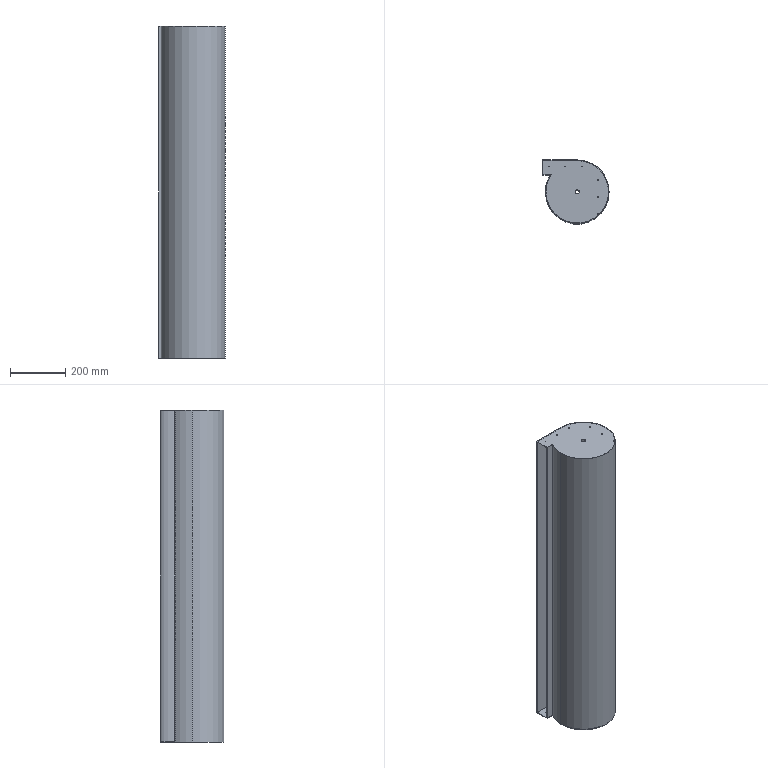Part | SolidWorks | features BaseBody 1 | 1 solid | 43 faces | box 239.936 x 230.88 x 1204 mm | volume 2000614 mm3 | cylinder 34 | plane 9 | commonest cylinder face diameters 3.455 x24 15 x4 226.88 x3 230.88 x3
STEP:
#1=CARTESIAN_POINT('',(74.043,-287.472,-1202.));
#2=VERTEX_POINT('',#1);
#3=CARTESIAN_POINT('',(56.063,-349.342,-1202.));
#4=VERTEX_POINT('',#3);
#5=CARTESIAN_POINT('',(171.503,-349.342,-1202.));
#6=DIRECTION('',(0.,0.,1.));
#7=DIRECTION('',(1.,0.,0.));
#8=AXIS2_PLACEMENT_3D('',#5,#6,#7);
#9=CIRCLE('',#8,115.44);
#10=EDGE_CURVE('',#2,#4,#9,.T.);
#11=ORIENTED_EDGE('',*,*,#10,.T.);
#12=CARTESIAN_POINT('',(56.063,-349.342,2.));
#13=VERTEX_POINT('',#12);
#14=CARTESIAN_POINT('',(56.063,-349.342,0.));
#15=DIRECTION('',(0.,0.,1.));
#16=VECTOR('',#15,1000.);
#17=LINE('',#14,#16);
#18=EDGE_CURVE('',#4,#13,#17,.T.);
#19=ORIENTED_EDGE('',*,*,#18,.T.);
#20=CARTESIAN_POINT('',(74.043,-287.472,2.));
#21=VERTEX_POINT('',#20);
#22=CARTESIAN_POINT('',(171.503,-349.342,2.));
#23=DIRECTION('',(0.,0.,-1.));
#24=DIRECTION('',(1.,0.,0.));
#25=AXIS2_PLACEMENT_3D('',#22,#23,#24);
#26=CIRCLE('',#25,115.44);
#27=EDGE_CURVE('',#13,#21,#26,.T.);
#28=ORIENTED_EDGE('',*,*,#27,.T.);
#29=CARTESIAN_POINT('',(74.043,-287.472,0.));
#30=DIRECTION('',(0.,0.,-1.));
#31=VECTOR('',#30,1000.);
#32=LINE('',#29,#31);
#33=EDGE_CURVE('',#21,#2,#32,.T.);
#34=ORIENTED_EDGE('',*,*,#33,.T.);
#35=EDGE_LOOP('',(#11,#19,#28,#34));
#36=FACE_OUTER_BOUND('',#35,.T.);
#37=CARTESIAN_POINT('',(171.503,-349.342,0.));
#38=DIRECTION('',(0.,0.,1.));
#39=DIRECTION('',(1.,0.,0.));
#40=AXIS2_PLACEMENT_3D('',#37,#38,#39);
#41=CYLINDRICAL_SURFACE('',#40,115.44);
#42=ADVANCED_FACE('',(#36),#41,.T.);
#43=ORIENTED_EDGE('',*,*,#18,.F.);
#44=CARTESIAN_POINT('',(286.943,-349.342,-1202.));
#45=VERTEX_POINT('',#44);
#46=CARTESIAN_POINT('',(171.503,-349.342,-1202.));
#47=DIRECTION('',(0.,0.,1.));
#48=DIRECTION('',(1.,0.,0.));
#49=AXIS2_PLACEMENT_3D('',#46,#47,#48);
#50=CIRCLE('',#49,115.44);
#51=EDGE_CURVE('',#4,#45,#50,.T.);
#52=ORIENTED_EDGE('',*,*,#51,.T.);
#53=CARTESIAN_POINT('',(286.943,-349.342,2.));
#54=VERTEX_POINT('',#53);
#55=CARTESIAN_POINT('',(286.943,-349.342,0.));
#56=DIRECTION('',(0.,0.,1.));
#57=VECTOR('',#56,1000.);
#58=LINE('',#55,#57);
#59=EDGE_CURVE('',#45,#54,#58,.T.);
#60=ORIENTED_EDGE('',*,*,#59,.T.);
#61=CARTESIAN_POINT('',(171.503,-349.342,2.));
#62=DIRECTION('',(0.,0.,-1.));
#63=DIRECTION('',(1.,0.,0.));
#64=AXIS2_PLACEMENT_3D('',#61,#62,#63);
#65=CIRCLE('',#64,115.44);
#66=EDGE_CURVE('',#54,#13,#65,.T.);
#67=ORIENTED_EDGE('',*,*,#66,.T.);
#68=EDGE_LOOP('',(#43,#52,#60,#67));
#69=FACE_OUTER_BOUND('',#68,.T.);
#70=CARTESIAN_POINT('',(171.503,-349.342,0.));
#71=DIRECTION('',(0.,0.,1.));
#72=DIRECTION('',(1.,0.,0.));
#73=AXIS2_PLACEMENT_3D('',#70,#71,#72);
#74=CYLINDRICAL_SURFACE('',#73,115.44);
#75=ADVANCED_FACE('',(#69),#74,.T.);
#76=CARTESIAN_POINT('',(179.003,-349.342,-1202.));
#77=VERTEX_POINT('',#76);
#78=CARTESIAN_POINT('',(164.003,-349.342,-1202.));
#79=VERTEX_POINT('',#78);
#80=CARTESIAN_POINT('',(171.503,-349.342,-1202.));
#81=DIRECTION('',(0.,0.,-1.));
#82=DIRECTION('',(1.,0.,0.));
#83=AXIS2_PLACEMENT_3D('',#80,#81,#82);
#84=CIRCLE('',#83,7.5);
#85=EDGE_CURVE('',#77,#79,#84,.T.);
#86=ORIENTED_EDGE('',*,*,#85,.T.);
#87=CARTESIAN_POINT('',(164.003,-349.342,-1200.));
#88=VERTEX_POINT('',#87);
#89=CARTESIAN_POINT('',(164.003,-349.342,-1202.));
#90=DIRECTION('',(0.,0.,1.));
#91=VECTOR('',#90,1000.);
#92=LINE('',#89,#91);
#93=EDGE_CURVE('',#79,#88,#92,.T.);
#94=ORIENTED_EDGE('',*,*,#93,.T.);
#95=CARTESIAN_POINT('',(179.003,-349.342,-1200.));
#96=VERTEX_POINT('',#95);
#97=CARTESIAN_POINT('',(171.503,-349.342,-1200.));
#98=DIRECTION('',(0.,0.,-1.));
#99=DIRECTION('',(1.,0.,0.));
#100=AXIS2_PLACEMENT_3D('',#97,#98,#99);
#101=CIRCLE('',#100,7.5);
#102=EDGE_CURVE('',#96,#88,#101,.T.);
#103=ORIENTED_EDGE('',*,*,#102,.F.);
#104=CARTESIAN_POINT('',(179.003,-349.342,-1202.));
#105=DIRECTION('',(0.,0.,1.));
#106=VECTOR('',#105,1000.);
#107=LINE('',#104,#106);
#108=EDGE_CURVE('',#77,#96,#107,.T.);
#109=ORIENTED_EDGE('',*,*,#108,.F.);
#110=EDGE_LOOP('',(#86,#94,#103,#109));
#111=FACE_OUTER_BOUND('',#110,.T.);
#112=CARTESIAN_POINT('',(171.503,-349.342,-1202.));
#113=DIRECTION('',(0.,0.,1.));
#114=DIRECTION('',(1.,0.,0.));
#115=AXIS2_PLACEMENT_3D('',#112,#113,#114);
#116=CYLINDRICAL_SURFACE('',#115,7.5);
#117=ADVANCED_FACE('',(#111),#116,.F.);
#118=CARTESIAN_POINT('',(248.518,-430.281,-1200.));
#119=VERTEX_POINT('',#118);
#120=CARTESIAN_POINT('',(245.063,-430.281,-1200.));
#121=VERTEX_POINT('',#120);
#122=CARTESIAN_POINT('',(246.79,-430.281,-1200.));
#123=DIRECTION('',(0.,0.,-1.));
#124=DIRECTION('',(-1.,0.,0.));
#125=AXIS2_PLACEMENT_3D('',#122,#123,#124);
#126=CIRCLE('',#125,1.728);
#127=EDGE_CURVE('',#119,#121,#126,.T.);
#128=ORIENTED_EDGE('',*,*,#127,.F.);
#129=CARTESIAN_POINT('',(248.518,-430.281,-1202.));
#130=VERTEX_POINT('',#129);
#131=CARTESIAN_POINT('',(248.518,-430.281,2.));
#132=DIRECTION('',(0.,0.,-1.));
#133=VECTOR('',#132,1000.);
#134=LINE('',#131,#133);
#135=EDGE_CURVE('',#119,#130,#134,.T.);
#136=ORIENTED_EDGE('',*,*,#135,.T.);
#137=CARTESIAN_POINT('',(245.063,-430.281,-1202.));
#138=VERTEX_POINT('',#137);
#139=CARTESIAN_POINT('',(246.79,-430.281,-1202.));
#140=DIRECTION('',(0.,0.,-1.));
#141=DIRECTION('',(-1.,0.,0.));
#142=AXIS2_PLACEMENT_3D('',#139,#140,#141);
#143=CIRCLE('',#142,1.728);
#144=EDGE_CURVE('',#130,#138,#143,.T.);
#145=ORIENTED_EDGE('',*,*,#144,.T.);
#146=CARTESIAN_POINT('',(245.063,-430.281,2.));
#147=DIRECTION('',(0.,0.,-1.));
#148=VECTOR('',#147,1000.);
#149=LINE('',#146,#148);
#150=EDGE_CURVE('',#121,#138,#149,.T.);
#151=ORIENTED_EDGE('',*,*,#150,.F.);
#152=EDGE_LOOP('',(#128,#136,#145,#151));
#153=FACE_OUTER_BOUND('',#152,.T.);
#154=CARTESIAN_POINT('',(246.79,-430.281,2.));
#155=DIRECTION('',(0.,0.,-1.));
#156=DIRECTION('',(-1.,0.,0.));
#157=AXIS2_PLACEMENT_3D('',#154,#155,#156);
#158=CYLINDRICAL_SURFACE('',#157,1.728);
#159=ADVANCED_FACE('',(#153),#158,.F.);
#160=CARTESIAN_POINT('',(248.518,-368.281,-1200.));
#161=VERTEX_POINT('',#160);
#162=CARTESIAN_POINT('',(245.063,-368.281,-1200.));
#163=VERTEX_POINT('',#162);
#164=CARTESIAN_POINT('',(246.79,-368.281,-1200.));
#165=DIRECTION('',(0.,0.,-1.));
#166=DIRECTION('',(-1.,0.,0.));
#167=AXIS2_PLACEMENT_3D('',#164,#165,#166);
#168=CIRCLE('',#167,1.728);
#169=EDGE_CURVE('',#161,#163,#168,.T.);
#170=ORIENTED_EDGE('',*,*,#169,.F.);
#171=CARTESIAN_POINT('',(248.518,-368.281,-1202.));
#172=VERTEX_POINT('',#171);
#173=CARTESIAN_POINT('',(248.518,-368.281,2.));
#174=DIRECTION('',(0.,0.,-1.));
#175=VECTOR('',#174,1000.);
#176=LINE('',#173,#175);
#177=EDGE_CURVE('',#161,#172,#176,.T.);
#178=ORIENTED_EDGE('',*,*,#177,.T.);
#179=CARTESIAN_POINT('',(245.063,-368.281,-1202.));
#180=VERTEX_POINT('',#179);
#181=CARTESIAN_POINT('',(246.79,-368.281,-1202.));
#182=DIRECTION('',(0.,0.,-1.));
#183=DIRECTION('',(-1.,0.,0.));
#184=AXIS2_PLACEMENT_3D('',#181,#182,#183);
#185=CIRCLE('',#184,1.728);
#186=EDGE_CURVE('',#172,#180,#185,.T.);
#187=ORIENTED_EDGE('',*,*,#186,.T.);
#188=CARTESIAN_POINT('',(245.063,-368.281,2.));
#189=DIRECTION('',(0.,0.,-1.));
#190=VECTOR('',#189,1000.);
#191=LINE('',#188,#190);
#192=EDGE_CURVE('',#163,#180,#191,.T.);
#193=ORIENTED_EDGE('',*,*,#192,.F.);
#194=EDGE_LOOP('',(#170,#178,#187,#193));
#195=FACE_OUTER_BOUND('',#194,.T.);
#196=CARTESIAN_POINT('',(246.79,-368.281,2.));
#197=DIRECTION('',(0.,0.,-1.));
#198=DIRECTION('',(-1.,0.,0.));
#199=AXIS2_PLACEMENT_3D('',#196,#197,#198);
#200=CYLINDRICAL_SURFACE('',#199,1.728);
#201=ADVANCED_FACE('',(#195),#200,.F.);
#202=CARTESIAN_POINT('',(130.294,-257.413,-1200.));
#203=VERTEX_POINT('',#202);
#204=CARTESIAN_POINT('',(126.839,-257.413,-1200.));
#205=VERTEX_POINT('',#204);
#206=CARTESIAN_POINT('',(128.567,-257.413,-1200.));
#207=DIRECTION('',(0.,0.,-1.));
#208=DIRECTION('',(-1.,0.,0.));
#209=AXIS2_PLACEMENT_3D('',#206,#207,#208);
#210=CIRCLE('',#209,1.728);
#211=EDGE_CURVE('',#203,#205,#210,.T.);
#212=ORIENTED_EDGE('',*,*,#211,.F.);
#213=CARTESIAN_POINT('',(130.294,-257.413,-1202.));
#214=VERTEX_POINT('',#213);
#215=CARTESIAN_POINT('',(130.294,-257.413,2.));
#216=DIRECTION('',(0.,0.,-1.));
#217=VECTOR('',#216,1000.);
#218=LINE('',#215,#217);
#219=EDGE_CURVE('',#203,#214,#218,.T.);
#220=ORIENTED_EDGE('',*,*,#219,.T.);
#221=CARTESIAN_POINT('',(126.839,-257.413,-1202.));
#222=VERTEX_POINT('',#221);
#223=CARTESIAN_POINT('',(128.567,-257.413,-1202.));
#224=DIRECTION('',(0.,0.,-1.));
#225=DIRECTION('',(-1.,0.,0.));
#226=AXIS2_PLACEMENT_3D('',#223,#224,#225);
#227=CIRCLE('',#226,1.728);
#228=EDGE_CURVE('',#214,#222,#227,.T.);
#229=ORIENTED_EDGE('',*,*,#228,.T.);
#230=CARTESIAN_POINT('',(126.839,-257.413,2.));
#231=DIRECTION('',(0.,0.,-1.));
#232=VECTOR('',#231,1000.);
#233=LINE('',#230,#232);
#234=EDGE_CURVE('',#205,#222,#233,.T.);
#235=ORIENTED_EDGE('',*,*,#234,.F.);
#236=EDGE_LOOP('',(#212,#220,#229,#235));
#237=FACE_OUTER_BOUND('',#236,.T.);
#238=CARTESIAN_POINT('',(128.567,-257.413,2.));
#239=DIRECTION('',(0.,0.,-1.));
#240=DIRECTION('',(-1.,0.,0.));
#241=AXIS2_PLACEMENT_3D('',#238,#239,#240);
#242=CYLINDRICAL_SURFACE('',#241,1.728);
#243=ADVANCED_FACE('',(#237),#242,.F.);
#244=CARTESIAN_POINT('',(190.294,-257.413,-1200.));
#245=VERTEX_POINT('',#244);
#246=CARTESIAN_POINT('',(186.839,-257.413,-1200.));
#247=VERTEX_POINT('',#246);
#248=CARTESIAN_POINT('',(188.567,-257.413,-1200.));
#249=DIRECTION('',(0.,0.,-1.));
#250=DIRECTION('',(-1.,0.,0.));
#251=AXIS2_PLACEMENT_3D('',#248,#249,#250);
#252=CIRCLE('',#251,1.728);
#253=EDGE_CURVE('',#245,#247,#252,.T.);
#254=ORIENTED_EDGE('',*,*,#253,.F.);
#255=CARTESIAN_POINT('',(190.294,-257.413,-1202.));
#256=VERTEX_POINT('',#255);
#257=CARTESIAN_POINT('',(190.294,-257.413,2.));
#258=DIRECTION('',(0.,0.,-1.));
#259=VECTOR('',#258,1000.);
#260=LINE('',#257,#259);
#261=EDGE_CURVE('',#245,#256,#260,.T.);
#262=ORIENTED_EDGE('',*,*,#261,.T.);
#263=CARTESIAN_POINT('',(186.839,-257.413,-1202.));
#264=VERTEX_POINT('',#263);
#265=CARTESIAN_POINT('',(188.567,-257.413,-1202.));
#266=DIRECTION('',(0.,0.,-1.));
#267=DIRECTION('',(-1.,0.,0.));
#268=AXIS2_PLACEMENT_3D('',#265,#266,#267);
#269=CIRCLE('',#268,1.728);
#270=EDGE_CURVE('',#256,#264,#269,.T.);
#271=ORIENTED_EDGE('',*,*,#270,.T.);
#272=CARTESIAN_POINT('',(186.839,-257.413,2.));
#273=DIRECTION('',(0.,0.,-1.));
#274=VECTOR('',#273,1000.);
#275=LINE('',#272,#274);
#276=EDGE_CURVE('',#247,#264,#275,.T.);
#277=ORIENTED_EDGE('',*,*,#276,.F.);
#278=EDGE_LOOP('',(#254,#262,#271,#277));
#279=FACE_OUTER_BOUND('',#278,.T.);
#280=CARTESIAN_POINT('',(188.567,-257.413,2.));
#281=DIRECTION('',(0.,0.,-1.));
#282=DIRECTION('',(-1.,0.,0.));
#283=AXIS2_PLACEMENT_3D('',#280,#281,#282);
#284=CYLINDRICAL_SURFACE('',#283,1.728);
#285=ADVANCED_FACE('',(#279),#284,.F.);
#286=CARTESIAN_POINT('',(70.294,-257.413,-1200.));
#287=VERTEX_POINT('',#286);
#288=CARTESIAN_POINT('',(66.839,-257.413,-1200.));
#289=VERTEX_POINT('',#288);
#290=CARTESIAN_POINT('',(68.567,-257.413,-1200.));
#291=DIRECTION('',(0.,0.,-1.));
#292=DIRECTION('',(-1.,0.,0.));
#293=AXIS2_PLACEMENT_3D('',#290,#291,#292);
#294=CIRCLE('',#293,1.728);
#295=EDGE_CURVE('',#287,#289,#294,.T.);
#296=ORIENTED_EDGE('',*,*,#295,.F.);
#297=CARTESIAN_POINT('',(70.294,-257.413,-1202.));
#298=VERTEX_POINT('',#297);
#299=CARTESIAN_POINT('',(70.294,-257.413,2.));
#300=DIRECTION('',(0.,0.,-1.));
#301=VECTOR('',#300,1000.);
#302=LINE('',#299,#301);
#303=EDGE_CURVE('',#287,#298,#302,.T.);
#304=ORIENTED_EDGE('',*,*,#303,.T.);
#305=CARTESIAN_POINT('',(66.839,-257.413,-1202.));
#306=VERTEX_POINT('',#305);
#307=CARTESIAN_POINT('',(68.567,-257.413,-1202.));
#308=DIRECTION('',(0.,0.,-1.));
#309=DIRECTION('',(-1.,0.,0.));
#310=AXIS2_PLACEMENT_3D('',#307,#308,#309);
#311=CIRCLE('',#310,1.728);
#312=EDGE_CURVE('',#298,#306,#311,.T.);
#313=ORIENTED_EDGE('',*,*,#312,.T.);
#314=CARTESIAN_POINT('',(66.839,-257.413,2.));
#315=DIRECTION('',(0.,0.,-1.));
#316=VECTOR('',#315,1000.);
#317=LINE('',#314,#316);
#318=EDGE_CURVE('',#289,#306,#317,.T.);
#319=ORIENTED_EDGE('',*,*,#318,.F.);
#320=EDGE_LOOP('',(#296,#304,#313,#319));
#321=FACE_OUTER_BOUND('',#320,.T.);
#322=CARTESIAN_POINT('',(68.567,-257.413,2.));
#323=DIRECTION('',(0.,0.,-1.));
#324=DIRECTION('',(-1.,0.,0.));
#325=AXIS2_PLACEMENT_3D('',#322,#323,#324);
#326=CYLINDRICAL_SURFACE('',#325,1.728);
#327=ADVANCED_FACE('',(#321),#326,.F.);
#328=CARTESIAN_POINT('',(248.518,-306.281,-1200.));
#329=VERTEX_POINT('',#328);
#330=CARTESIAN_POINT('',(245.063,-306.281,-1200.));
#331=VERTEX_POINT('',#330);
#332=CARTESIAN_POINT('',(246.79,-306.281,-1200.));
#333=DIRECTION('',(0.,0.,-1.));
#334=DIRECTION('',(-1.,0.,0.));
#335=AXIS2_PLACEMENT_3D('',#332,#333,#334);
#336=CIRCLE('',#335,1.728);
#337=EDGE_CURVE('',#329,#331,#336,.T.);
#338=ORIENTED_EDGE('',*,*,#337,.F.);
#339=CARTESIAN_POINT('',(248.518,-306.281,-1202.));
#340=VERTEX_POINT('',#339);
#341=CARTESIAN_POINT('',(248.518,-306.281,2.));
#342=DIRECTION('',(0.,0.,-1.));
#343=VECTOR('',#342,1000.);
#344=LINE('',#341,#343);
#345=EDGE_CURVE('',#329,#340,#344,.T.);
#346=ORIENTED_EDGE('',*,*,#345,.T.);
#347=CARTESIAN_POINT('',(245.063,-306.281,-1202.));
#348=VERTEX_POINT('',#347);
#349=CARTESIAN_POINT('',(246.79,-306.281,-1202.));
#350=DIRECTION('',(0.,0.,-1.));
#351=DIRECTION('',(-1.,0.,0.));
#352=AXIS2_PLACEMENT_3D('',#349,#350,#351);
#353=CIRCLE('',#352,1.728);
#354=EDGE_CURVE('',#340,#348,#353,.T.);
#355=ORIENTED_EDGE('',*,*,#354,.T.);
#356=CARTESIAN_POINT('',(245.063,-306.281,2.));
#357=DIRECTION('',(0.,0.,-1.));
#358=VECTOR('',#357,1000.);
#359=LINE('',#356,#358);
#360=EDGE_CURVE('',#331,#348,#359,.T.);
#361=ORIENTED_EDGE('',*,*,#360,.F.);
#362=EDGE_LOOP('',(#338,#346,#355,#361));
#363=FACE_OUTER_BOUND('',#362,.T.);
#364=CARTESIAN_POINT('',(246.79,-306.281,2.));
#365=DIRECTION('',(0.,0.,-1.));
#366=DIRECTION('',(-1.,0.,0.));
#367=AXIS2_PLACEMENT_3D('',#364,#365,#366);
#368=CYLINDRICAL_SURFACE('',#367,1.728);
#369=ADVANCED_FACE('',(#363),#368,.F.);
#370=CARTESIAN_POINT('',(164.003,-349.342,0.));
#371=VERTEX_POINT('',#370);
#372=CARTESIAN_POINT('',(179.003,-349.342,0.));
#373=VERTEX_POINT('',#372);
#374=CARTESIAN_POINT('',(171.503,-349.342,0.));
#375=DIRECTION('',(0.,0.,1.));
#376=DIRECTION('',(1.,0.,0.));
#377=AXIS2_PLACEMENT_3D('',#374,#375,#376);
#378=CIRCLE('',#377,7.5);
#379=EDGE_CURVE('',#371,#373,#378,.T.);
#380=ORIENTED_EDGE('',*,*,#379,.F.);
#381=CARTESIAN_POINT('',(164.003,-349.342,2.));
#382=VERTEX_POINT('',#381);
#383=CARTESIAN_POINT('',(164.003,-349.342,0.));
#384=DIRECTION('',(0.,0.,1.));
#385=VECTOR('',#384,1000.);
#386=LINE('',#383,#385);
#387=EDGE_CURVE('',#371,#382,#386,.T.);
#388=ORIENTED_EDGE('',*,*,#387,.T.);
#389=CARTESIAN_POINT('',(179.003,-349.342,2.));
#390=VERTEX_POINT('',#389);
#391=CARTESIAN_POINT('',(171.503,-349.342,2.));
#392=DIRECTION('',(0.,0.,-1.));
#393=DIRECTION('',(1.,0.,0.));
#394=AXIS2_PLACEMENT_3D('',#391,#392,#393);
#395=CIRCLE('',#394,7.5);
#396=EDGE_CURVE('',#390,#382,#395,.T.);
#397=ORIENTED_EDGE('',*,*,#396,.F.);
#398=CARTESIAN_POINT('',(179.003,-349.342,0.));
#399=DIRECTION('',(0.,0.,1.));
#400=VECTOR('',#399,1000.);
#401=LINE('',#398,#400);
#402=EDGE_CURVE('',#373,#390,#401,.T.);
#403=ORIENTED_EDGE('',*,*,#402,.F.);
#404=EDGE_LOOP('',(#380,#388,#397,#403));
#405=FACE_OUTER_BOUND('',#404,.T.);
#406=CARTESIAN_POINT('',(171.503,-349.342,0.));
#407=DIRECTION('',(0.,0.,1.));
#408=DIRECTION('',(1.,0.,0.));
#409=AXIS2_PLACEMENT_3D('',#406,#407,#408);
#410=CYLINDRICAL_SURFACE('',#409,7.5);
#411=ADVANCED_FACE('',(#405),#410,.F.);
#412=CARTESIAN_POINT('',(248.518,-430.281,2.));
#413=VERTEX_POINT('',#412);
#414=CARTESIAN_POINT('',(245.063,-430.281,2.));
#415=VERTEX_POINT('',#414);
#416=CARTESIAN_POINT('',(246.79,-430.281,2.));
#417=DIRECTION('',(0.,0.,-1.));
#418=DIRECTION('',(-1.,0.,0.));
#419=AXIS2_PLACEMENT_3D('',#416,#417,#418);
#420=CIRCLE('',#419,1.728);
#421=EDGE_CURVE('',#413,#415,#420,.T.);
#422=ORIENTED_EDGE('',*,*,#421,.F.);
#423=CARTESIAN_POINT('',(248.518,-430.281,0.));
#424=VERTEX_POINT('',#423);
#425=CARTESIAN_POINT('',(248.518,-430.281,2.));
#426=DIRECTION('',(0.,0.,-1.));
#427=VECTOR('',#426,1000.);
#428=LINE('',#425,#427);
#429=EDGE_CURVE('',#413,#424,#428,.T.);
#430=ORIENTED_EDGE('',*,*,#429,.T.);
#431=CARTESIAN_POINT('',(245.063,-430.281,0.));
#432=VERTEX_POINT('',#431);
#433=CARTESIAN_POINT('',(246.79,-430.281,0.));
#434=DIRECTION('',(0.,0.,1.));
#435=DIRECTION('',(-1.,0.,0.));
#436=AXIS2_PLACEMENT_3D('',#433,#434,#435);
#437=CIRCLE('',#436,1.728);
#438=EDGE_CURVE('',#432,#424,#437,.T.);
#439=ORIENTED_EDGE('',*,*,#438,.F.);
#440=CARTESIAN_POINT('',(245.063,-430.281,2.));
#441=DIRECTION('',(0.,0.,-1.));
#442=VECTOR('',#441,1000.);
#443=LINE('',#440,#442);
#444=EDGE_CURVE('',#415,#432,#443,.T.);
#445=ORIENTED_EDGE('',*,*,#444,.F.);
#446=EDGE_LOOP('',(#422,#430,#439,#445));
#447=FACE_OUTER_BOUND('',#446,.T.);
#448=CARTESIAN_POINT('',(246.79,-430.281,2.));
#449=DIRECTION('',(0.,0.,-1.));
#450=DIRECTION('',(-1.,0.,0.));
#451=AXIS2_PLACEMENT_3D('',#448,#449,#450);
#452=CYLINDRICAL_SURFACE('',#451,1.728);
#453=ADVANCED_FACE('',(#447),#452,.F.);
#454=CARTESIAN_POINT('',(248.518,-368.281,2.));
#455=VERTEX_POINT('',#454);
#456=CARTESIAN_POINT('',(245.063,-368.281,2.));
#457=VERTEX_POINT('',#456);
#458=CARTESIAN_POINT('',(246.79,-368.281,2.));
#459=DIRECTION('',(0.,0.,-1.));
#460=DIRECTION('',(-1.,0.,0.));
#461=AXIS2_PLACEMENT_3D('',#458,#459,#460);
#462=CIRCLE('',#461,1.728);
#463=EDGE_CURVE('',#455,#457,#462,.T.);
#464=ORIENTED_EDGE('',*,*,#463,.F.);
#465=CARTESIAN_POINT('',(248.518,-368.281,0.));
#466=VERTEX_POINT('',#465);
#467=CARTESIAN_POINT('',(248.518,-368.281,2.));
#468=DIRECTION('',(0.,0.,-1.));
#469=VECTOR('',#468,1000.);
#470=LINE('',#467,#469);
#471=EDGE_CURVE('',#455,#466,#470,.T.);
#472=ORIENTED_EDGE('',*,*,#471,.T.);
#473=CARTESIAN_POINT('',(245.063,-368.281,0.));
#474=VERTEX_POINT('',#473);
#475=CARTESIAN_POINT('',(246.79,-368.281,0.));
#476=DIRECTION('',(0.,0.,1.));
#477=DIRECTION('',(-1.,0.,0.));
#478=AXIS2_PLACEMENT_3D('',#475,#476,#477);
#479=CIRCLE('',#478,1.728);
#480=EDGE_CURVE('',#474,#466,#479,.T.);
#481=ORIENTED_EDGE('',*,*,#480,.F.);
#482=CARTESIAN_POINT('',(245.063,-368.281,2.));
#483=DIRECTION('',(0.,0.,-1.));
#484=VECTOR('',#483,1000.);
#485=LINE('',#482,#484);
#486=EDGE_CURVE('',#457,#474,#485,.T.);
#487=ORIENTED_EDGE('',*,*,#486,.F.);
#488=EDGE_LOOP('',(#464,#472,#481,#487));
#489=FACE_OUTER_BOUND('',#488,.T.);
#490=CARTESIAN_POINT('',(246.79,-368.281,2.));
#491=DIRECTION('',(0.,0.,-1.));
#492=DIRECTION('',(-1.,0.,0.));
#493=AXIS2_PLACEMENT_3D('',#490,#491,#492);
#494=CYLINDRICAL_SURFACE('',#493,1.728);
#495=ADVANCED_FACE('',(#489),#494,.F.);
#496=CARTESIAN_POINT('',(130.294,-257.413,2.));
#497=VERTEX_POINT('',#496);
#498=CARTESIAN_POINT('',(126.839,-257.413,2.));
#499=VERTEX_POINT('',#498);
#500=CARTESIAN_POINT('',(128.567,-257.413,2.));
#501=DIRECTION('',(0.,0.,-1.));
#502=DIRECTION('',(-1.,0.,0.));
#503=AXIS2_PLACEMENT_3D('',#500,#501,#502);
#504=CIRCLE('',#503,1.728);
#505=EDGE_CURVE('',#497,#499,#504,.T.);
#506=ORIENTED_EDGE('',*,*,#505,.F.);
#507=CARTESIAN_POINT('',(130.294,-257.413,0.));
#508=VERTEX_POINT('',#507);
#509=CARTESIAN_POINT('',(130.294,-257.413,2.));
#510=DIRECTION('',(0.,0.,-1.));
#511=VECTOR('',#510,1000.);
#512=LINE('',#509,#511);
#513=EDGE_CURVE('',#497,#508,#512,.T.);
#514=ORIENTED_EDGE('',*,*,#513,.T.);
#515=CARTESIAN_POINT('',(126.839,-257.413,0.));
#516=VERTEX_POINT('',#515);
#517=CARTESIAN_POINT('',(128.567,-257.413,0.));
#518=DIRECTION('',(0.,0.,1.));
#519=DIRECTION('',(-1.,0.,0.));
#520=AXIS2_PLACEMENT_3D('',#517,#518,#519);
#521=CIRCLE('',#520,1.728);
#522=EDGE_CURVE('',#516,#508,#521,.T.);
#523=ORIENTED_EDGE('',*,*,#522,.F.);
#524=CARTESIAN_POINT('',(126.839,-257.413,2.));
#525=DIRECTION('',(0.,0.,-1.));
#526=VECTOR('',#525,1000.);
#527=LINE('',#524,#526);
#528=EDGE_CURVE('',#499,#516,#527,.T.);
#529=ORIENTED_EDGE('',*,*,#528,.F.);
#530=EDGE_LOOP('',(#506,#514,#523,#529));
#531=FACE_OUTER_BOUND('',#530,.T.);
#532=CARTESIAN_POINT('',(128.567,-257.413,2.));
#533=DIRECTION('',(0.,0.,-1.));
#534=DIRECTION('',(-1.,0.,0.));
#535=AXIS2_PLACEMENT_3D('',#532,#533,#534);
#536=CYLINDRICAL_SURFACE('',#535,1.728);
#537=ADVANCED_FACE('',(#531),#536,.F.);
#538=CARTESIAN_POINT('',(190.294,-257.413,2.));
#539=VERTEX_POINT('',#538);
#540=CARTESIAN_POINT('',(186.839,-257.413,2.));
#541=VERTEX_POINT('',#540);
#542=CARTESIAN_POINT('',(188.567,-257.413,2.));
#543=DIRECTION('',(0.,0.,-1.));
#544=DIRECTION('',(-1.,0.,0.));
#545=AXIS2_PLACEMENT_3D('',#542,#543,#544);
#546=CIRCLE('',#545,1.728);
#547=EDGE_CURVE('',#539,#541,#546,.T.);
#548=ORIENTED_EDGE('',*,*,#547,.F.);
#549=CARTESIAN_POINT('',(190.294,-257.413,0.));
#550=VERTEX_POINT('',#549);
#551=CARTESIAN_POINT('',(190.294,-257.413,2.));
#552=DIRECTION('',(0.,0.,-1.));
#553=VECTOR('',#552,1000.);
#554=LINE('',#551,#553);
#555=EDGE_CURVE('',#539,#550,#554,.T.);
#556=ORIENTED_EDGE('',*,*,#555,.T.);
#557=CARTESIAN_POINT('',(186.839,-257.413,0.));
#558=VERTEX_POINT('',#557);
#559=CARTESIAN_POINT('',(188.567,-257.413,0.));
#560=DIRECTION('',(0.,0.,1.));
#561=DIRECTION('',(-1.,0.,0.));
#562=AXIS2_PLACEMENT_3D('',#559,#560,#561);
#563=CIRCLE('',#562,1.728);
#564=EDGE_CURVE('',#558,#550,#563,.T.);
#565=ORIENTED_EDGE('',*,*,#564,.F.);
#566=CARTESIAN_POINT('',(186.839,-257.413,2.));
#567=DIRECTION('',(0.,0.,-1.));
#568=VECTOR('',#567,1000.);
#569=LINE('',#566,#568);
#570=EDGE_CURVE('',#541,#558,#569,.T.);
#571=ORIENTED_EDGE('',*,*,#570,.F.);
#572=EDGE_LOOP('',(#548,#556,#565,#571));
#573=FACE_OUTER_BOUND('',#572,.T.);
#574=CARTESIAN_POINT('',(188.567,-257.413,2.));
#575=DIRECTION('',(0.,0.,-1.));
#576=DIRECTION('',(-1.,0.,0.));
#577=AXIS2_PLACEMENT_3D('',#574,#575,#576);
#578=CYLINDRICAL_SURFACE('',#577,1.728);
#579=ADVANCED_FACE('',(#573),#578,.F.);
#580=CARTESIAN_POINT('',(70.294,-257.413,2.));
#581=VERTEX_POINT('',#580);
#582=CARTESIAN_POINT('',(66.839,-257.413,2.));
#583=VERTEX_POINT('',#582);
#584=CARTESIAN_POINT('',(68.567,-257.413,2.));
#585=DIRECTION('',(0.,0.,-1.));
#586=DIRECTION('',(-1.,0.,0.));
#587=AXIS2_PLACEMENT_3D('',#584,#585,#586);
#588=CIRCLE('',#587,1.728);
#589=EDGE_CURVE('',#581,#583,#588,.T.);
#590=ORIENTED_EDGE('',*,*,#589,.F.);
#591=CARTESIAN_POINT('',(70.294,-257.413,0.));
#592=VERTEX_POINT('',#591);
#593=CARTESIAN_POINT('',(70.294,-257.413,2.));
#594=DIRECTION('',(0.,0.,-1.));
#595=VECTOR('',#594,1000.);
#596=LINE('',#593,#595);
#597=EDGE_CURVE('',#581,#592,#596,.T.);
#598=ORIENTED_EDGE('',*,*,#597,.T.);
#599=CARTESIAN_POINT('',(66.839,-257.413,0.));
#600=VERTEX_POINT('',#599);
#601=CARTESIAN_POINT('',(68.567,-257.413,0.));
#602=DIRECTION('',(0.,0.,1.));
#603=DIRECTION('',(-1.,0.,0.));
#604=AXIS2_PLACEMENT_3D('',#601,#602,#603);
#605=CIRCLE('',#604,1.728);
#606=EDGE_CURVE('',#600,#592,#605,.T.);
#607=ORIENTED_EDGE('',*,*,#606,.F.);
#608=CARTESIAN_POINT('',(66.839,-257.413,2.));
#609=DIRECTION('',(0.,0.,-1.));
#610=VECTOR('',#609,1000.);
#611=LINE('',#608,#610);
#612=EDGE_CURVE('',#583,#600,#611,.T.);
#613=ORIENTED_EDGE('',*,*,#612,.F.);
#614=EDGE_LOOP('',(#590,#598,#607,#613));
#615=FACE_OUTER_BOUND('',#614,.T.);
#616=CARTESIAN_POINT('',(68.567,-257.413,2.));
#617=DIRECTION('',(0.,0.,-1.));
#618=DIRECTION('',(-1.,0.,0.));
#619=AXIS2_PLACEMENT_3D('',#616,#617,#618);
#620=CYLINDRICAL_SURFACE('',#619,1.728);
#621=ADVANCED_FACE('',(#615),#620,.F.);
#622=CARTESIAN_POINT('',(248.518,-306.281,2.));
#623=VERTEX_POINT('',#622);
#624=CARTESIAN_POINT('',(245.063,-306.281,2.));
#625=VERTEX_POINT('',#624);
#626=CARTESIAN_POINT('',(246.79,-306.281,2.));
#627=DIRECTION('',(0.,0.,-1.));
#628=DIRECTION('',(-1.,0.,0.));
#629=AXIS2_PLACEMENT_3D('',#626,#627,#628);
#630=CIRCLE('',#629,1.728);
#631=EDGE_CURVE('',#623,#625,#630,.T.);
#632=ORIENTED_EDGE('',*,*,#631,.F.);
#633=CARTESIAN_POINT('',(248.518,-306.281,0.));
#634=VERTEX_POINT('',#633);
#635=CARTESIAN_POINT('',(248.518,-306.281,2.));
#636=DIRECTION('',(0.,0.,-1.));
#637=VECTOR('',#636,1000.);
#638=LINE('',#635,#637);
#639=EDGE_CURVE('',#623,#634,#638,.T.);
#640=ORIENTED_EDGE('',*,*,#639,.T.);
#641=CARTESIAN_POINT('',(245.063,-306.281,0.));
#642=VERTEX_POINT('',#641);
#643=CARTESIAN_POINT('',(246.79,-306.281,0.));
#644=DIRECTION('',(0.,0.,1.));
#645=DIRECTION('',(-1.,0.,0.));
#646=AXIS2_PLACEMENT_3D('',#643,#644,#645);
#647=CIRCLE('',#646,1.728);
#648=EDGE_CURVE('',#642,#634,#647,.T.);
#649=ORIENTED_EDGE('',*,*,#648,.F.);
#650=CARTESIAN_POINT('',(245.063,-306.281,2.));
#651=DIRECTION('',(0.,0.,-1.));
#652=VECTOR('',#651,1000.);
#653=LINE('',#650,#652);
#654=EDGE_CURVE('',#625,#642,#653,.T.);
#655=ORIENTED_EDGE('',*,*,#654,.F.);
#656=EDGE_LOOP('',(#632,#640,#649,#655));
#657=FACE_OUTER_BOUND('',#656,.T.);
#658=CARTESIAN_POINT('',(246.79,-306.281,2.));
#659=DIRECTION('',(0.,0.,-1.));
#660=DIRECTION('',(-1.,0.,0.));
#661=AXIS2_PLACEMENT_3D('',#658,#659,#660);
#662=CYLINDRICAL_SURFACE('',#661,1.728);
#663=ADVANCED_FACE('',(#657),#662,.F.);
#664=CARTESIAN_POINT('',(58.063,-349.342,-1200.));
#665=VERTEX_POINT('',#664);
#666=CARTESIAN_POINT('',(284.943,-349.342,-1200.));
#667=VERTEX_POINT('',#666);
#668=CARTESIAN_POINT('',(171.503,-349.342,-1200.));
#669=DIRECTION('',(0.,0.,1.));
#670=DIRECTION('',(1.,0.,0.));
#671=AXIS2_PLACEMENT_3D('',#668,#669,#670);
#672=CIRCLE('',#671,113.44);
#673=EDGE_CURVE('',#665,#667,#672,.T.);
#674=ORIENTED_EDGE('',*,*,#673,.F.);
#675=CARTESIAN_POINT('',(58.063,-349.342,0.));
#676=VERTEX_POINT('',#675);
#677=CARTESIAN_POINT('',(58.063,-349.342,-1200.));
#678=DIRECTION('',(0.,0.,1.));
#679=VECTOR('',#678,1000.);
#680=LINE('',#677,#679);
#681=EDGE_CURVE('',#665,#676,#680,.T.);
#682=ORIENTED_EDGE('',*,*,#681,.T.);
#683=CARTESIAN_POINT('',(284.943,-349.342,0.));
#684=VERTEX_POINT('',#683);
#685=CARTESIAN_POINT('',(171.503,-349.342,0.));
#686=DIRECTION('',(0.,0.,1.));
#687=DIRECTION('',(1.,0.,0.));
#688=AXIS2_PLACEMENT_3D('',#685,#686,#687);
#689=CIRCLE('',#688,113.44);
#690=EDGE_CURVE('',#676,#684,#689,.T.);
#691=ORIENTED_EDGE('',*,*,#690,.T.);
#692=CARTESIAN_POINT('',(284.943,-349.342,-1200.));
#693=DIRECTION('',(0.,0.,1.));
#694=VECTOR('',#693,1000.);
#695=LINE('',#692,#694);
#696=EDGE_CURVE('',#667,#684,#695,.T.);
#697=ORIENTED_EDGE('',*,*,#696,.F.);
#698=EDGE_LOOP('',(#674,#682,#691,#697));
#699=FACE_OUTER_BOUND('',#698,.T.);
#700=CARTESIAN_POINT('',(171.503,-349.342,-1200.));
#701=DIRECTION('',(0.,0.,1.));
#702=DIRECTION('',(1.,0.,0.));
#703=AXIS2_PLACEMENT_3D('',#700,#701,#702);
#704=CYLINDRICAL_SURFACE('',#703,113.44);
#705=ADVANCED_FACE('',(#699),#704,.F.);
#706=CARTESIAN_POINT('',(171.503,-235.902,-1200.));
#707=VERTEX_POINT('',#706);
#708=CARTESIAN_POINT('',(171.503,-349.342,-1200.));
#709=DIRECTION('',(0.,0.,1.));
#710=DIRECTION('',(1.,0.,0.));
#711=AXIS2_PLACEMENT_3D('',#708,#709,#710);
#712=CIRCLE('',#711,113.44);
#713=EDGE_CURVE('',#667,#707,#712,.T.);
#714=ORIENTED_EDGE('',*,*,#713,.F.);
#715=ORIENTED_EDGE('',*,*,#696,.T.);
#716=CARTESIAN_POINT('',(171.503,-235.902,0.));
#717=VERTEX_POINT('',#716);
#718=CARTESIAN_POINT('',(171.503,-349.342,0.));
#719=DIRECTION('',(0.,0.,1.));
#720=DIRECTION('',(1.,0.,0.));
#721=AXIS2_PLACEMENT_3D('',#718,#719,#720);
#722=CIRCLE('',#721,113.44);
#723=EDGE_CURVE('',#684,#717,#722,.T.);
#724=ORIENTED_EDGE('',*,*,#723,.T.);
#725=CARTESIAN_POINT('',(171.503,-235.902,-1200.));
#726=DIRECTION('',(0.,0.,1.));
#727=VECTOR('',#726,1000.);
#728=LINE('',#725,#727);
#729=EDGE_CURVE('',#707,#717,#728,.T.);
#730=ORIENTED_EDGE('',*,*,#729,.F.);
#731=EDGE_LOOP('',(#714,#715,#724,#730));
#732=FACE_OUTER_BOUND('',#731,.T.);
#733=CARTESIAN_POINT('',(171.503,-349.342,-1200.));
#734=DIRECTION('',(0.,0.,1.));
#735=DIRECTION('',(1.,0.,0.));
#736=AXIS2_PLACEMENT_3D('',#733,#734,#735);
#737=CYLINDRICAL_SURFACE('',#736,113.44);
#738=ADVANCED_FACE('',(#732),#737,.F.);
#739=ORIENTED_EDGE('',*,*,#59,.F.);
#740=CARTESIAN_POINT('',(171.503,-233.902,-1202.));
#741=VERTEX_POINT('',#740);
#742=CARTESIAN_POINT('',(171.503,-349.342,-1202.));
#743=DIRECTION('',(0.,0.,1.));
#744=DIRECTION('',(1.,0.,0.));
#745=AXIS2_PLACEMENT_3D('',#742,#743,#744);
#746=CIRCLE('',#745,115.44);
#747=EDGE_CURVE('',#45,#741,#746,.T.);
#748=ORIENTED_EDGE('',*,*,#747,.T.);
#749=CARTESIAN_POINT('',(171.503,-233.902,2.));
#750=VERTEX_POINT('',#749);
#751=CARTESIAN_POINT('',(171.503,-233.902,0.));
#752=DIRECTION('',(0.,0.,1.));
#753=VECTOR('',#752,1000.);
#754=LINE('',#751,#753);
#755=EDGE_CURVE('',#741,#750,#754,.T.);
#756=ORIENTED_EDGE('',*,*,#755,.T.);
#757=CARTESIAN_POINT('',(171.503,-349.342,2.));
#758=DIRECTION('',(0.,0.,-1.));
#759=DIRECTION('',(1.,0.,0.));
#760=AXIS2_PLACEMENT_3D('',#757,#758,#759);
#761=CIRCLE('',#760,115.44);
#762=EDGE_CURVE('',#750,#54,#761,.T.);
#763=ORIENTED_EDGE('',*,*,#762,.T.);
#764=EDGE_LOOP('',(#739,#748,#756,#763));
#765=FACE_OUTER_BOUND('',#764,.T.);
#766=CARTESIAN_POINT('',(171.503,-349.342,0.));
#767=DIRECTION('',(0.,0.,1.));
#768=DIRECTION('',(1.,0.,0.));
#769=AXIS2_PLACEMENT_3D('',#766,#767,#768);
#770=CYLINDRICAL_SURFACE('',#769,115.44);
#771=ADVANCED_FACE('',(#765),#770,.T.);
#772=ORIENTED_EDGE('',*,*,#85,.F.);
#773=CARTESIAN_POINT('',(171.503,-349.342,-1202.));
#774=DIRECTION('',(0.,0.,-1.));
#775=DIRECTION('',(1.,0.,0.));
#776=AXIS2_PLACEMENT_3D('',#773,#774,#775);
#777=CIRCLE('',#776,7.5);
#778=EDGE_CURVE('',#79,#77,#777,.T.);
#779=ORIENTED_EDGE('',*,*,#778,.F.);
#780=EDGE_LOOP('',(#772,#779));
#781=FACE_BOUND('',#780,.T.);
#782=CARTESIAN_POINT('',(246.79,-430.281,-1202.));
#783=DIRECTION('',(0.,0.,-1.));
#784=DIRECTION('',(-1.,0.,0.));
#785=AXIS2_PLACEMENT_3D('',#782,#783,#784);
#786=CIRCLE('',#785,1.728);
#787=EDGE_CURVE('',#138,#130,#786,.T.);
#788=ORIENTED_EDGE('',*,*,#787,.F.);
#789=ORIENTED_EDGE('',*,*,#144,.F.);
#790=EDGE_LOOP('',(#788,#789));
#791=FACE_BOUND('',#790,.T.);
#792=CARTESIAN_POINT('',(246.79,-368.281,-1202.));
#793=DIRECTION('',(0.,0.,-1.));
#794=DIRECTION('',(-1.,0.,0.));
#795=AXIS2_PLACEMENT_3D('',#792,#793,#794);
#796=CIRCLE('',#795,1.728);
#797=EDGE_CURVE('',#180,#172,#796,.T.);
#798=ORIENTED_EDGE('',*,*,#797,.F.);
#799=ORIENTED_EDGE('',*,*,#186,.F.);
#800=EDGE_LOOP('',(#798,#799));
#801=FACE_BOUND('',#800,.T.);
#802=CARTESIAN_POINT('',(128.567,-257.413,-1202.));
#803=DIRECTION('',(0.,0.,-1.));
#804=DIRECTION('',(-1.,0.,0.));
#805=AXIS2_PLACEMENT_3D('',#802,#803,#804);
#806=CIRCLE('',#805,1.728);
#807=EDGE_CURVE('',#222,#214,#806,.T.);
#808=ORIENTED_EDGE('',*,*,#807,.F.);
#809=ORIENTED_EDGE('',*,*,#228,.F.);
#810=EDGE_LOOP('',(#808,#809));
#811=FACE_BOUND('',#810,.T.);
#812=CARTESIAN_POINT('',(188.567,-257.413,-1202.));
#813=DIRECTION('',(0.,0.,-1.));
#814=DIRECTION('',(-1.,0.,0.));
#815=AXIS2_PLACEMENT_3D('',#812,#813,#814);
#816=CIRCLE('',#815,1.728);
#817=EDGE_CURVE('',#264,#256,#816,.T.);
#818=ORIENTED_EDGE('',*,*,#817,.F.);
#819=ORIENTED_EDGE('',*,*,#270,.F.);
#820=EDGE_LOOP('',(#818,#819));
#821=FACE_BOUND('',#820,.T.);
#822=CARTESIAN_POINT('',(68.567,-257.413,-1202.));
#823=DIRECTION('',(0.,0.,-1.));
#824=DIRECTION('',(-1.,0.,0.));
#825=AXIS2_PLACEMENT_3D('',#822,#823,#824);
#826=CIRCLE('',#825,1.728);
#827=EDGE_CURVE('',#306,#298,#826,.T.);
#828=ORIENTED_EDGE('',*,*,#827,.F.);
#829=ORIENTED_EDGE('',*,*,#312,.F.);
#830=EDGE_LOOP('',(#828,#829));
#831=FACE_BOUND('',#830,.T.);
#832=CARTESIAN_POINT('',(246.79,-306.281,-1202.));
#833=DIRECTION('',(0.,0.,-1.));
#834=DIRECTION('',(-1.,0.,0.));
#835=AXIS2_PLACEMENT_3D('',#832,#833,#834);
#836=CIRCLE('',#835,1.728);
#837=EDGE_CURVE('',#348,#340,#836,.T.);
#838=ORIENTED_EDGE('',*,*,#837,.F.);
#839=ORIENTED_EDGE('',*,*,#354,.F.);
#840=EDGE_LOOP('',(#838,#839));
#841=FACE_BOUND('',#840,.T.);
#842=CARTESIAN_POINT('',(47.007,-233.902,-1202.));
#843=VERTEX_POINT('',#842);
#844=CARTESIAN_POINT('',(47.007,-287.472,-1202.));
#845=VERTEX_POINT('',#844);
#846=CARTESIAN_POINT('',(47.007,-349.342,-1202.));
#847=DIRECTION('',(0.,-1.,0.));
#848=VECTOR('',#847,1000.);
#849=LINE('',#846,#848);
#850=EDGE_CURVE('',#843,#845,#849,.T.);
#851=ORIENTED_EDGE('',*,*,#850,.F.);
#852=CARTESIAN_POINT('',(166.975,-233.902,-1202.));
#853=DIRECTION('',(-1.,0.,0.));
#854=VECTOR('',#853,1000.);
#855=LINE('',#852,#854);
#856=EDGE_CURVE('',#741,#843,#855,.T.);
#857=ORIENTED_EDGE('',*,*,#856,.F.);
#858=ORIENTED_EDGE('',*,*,#747,.F.);
#859=ORIENTED_EDGE('',*,*,#51,.F.);
#860=ORIENTED_EDGE('',*,*,#10,.F.);
#861=CARTESIAN_POINT('',(166.975,-287.472,-1202.));
#862=DIRECTION('',(1.,0.,0.));
#863=VECTOR('',#862,1000.);
#864=LINE('',#861,#863);
#865=EDGE_CURVE('',#845,#2,#864,.T.);
#866=ORIENTED_EDGE('',*,*,#865,.F.);
#867=EDGE_LOOP('',(#851,#857,#858,#859,#860,#866));
#868=FACE_OUTER_BOUND('',#867,.T.);
#869=CARTESIAN_POINT('',(166.975,-349.342,-1202.));
#870=DIRECTION('',(0.,0.,1.));
#871=DIRECTION('',(1.,0.,0.));
#872=AXIS2_PLACEMENT_3D('',#869,#870,#871);
#873=PLANE('',#872);
#874=ADVANCED_FACE('',(#781,#791,#801,#811,#821,#831,#841,#868),#873,.F.);
#875=CARTESIAN_POINT('',(47.007,-287.472,2.));
#876=VERTEX_POINT('',#875);
#877=CARTESIAN_POINT('',(47.007,-287.472,0.));
#878=DIRECTION('',(0.,0.,-1.));
#879=VECTOR('',#878,1000.);
#880=LINE('',#877,#879);
#881=EDGE_CURVE('',#876,#845,#880,.T.);
#882=ORIENTED_EDGE('',*,*,#881,.T.);
#883=ORIENTED_EDGE('',*,*,#865,.T.);
#884=ORIENTED_EDGE('',*,*,#33,.F.);
#885=CARTESIAN_POINT('',(47.007,-287.472,2.));
#886=DIRECTION('',(-1.,0.,0.));
#887=VECTOR('',#886,1000.);
#888=LINE('',#885,#887);
#889=EDGE_CURVE('',#21,#876,#888,.T.);
#890=ORIENTED_EDGE('',*,*,#889,.T.);
#891=EDGE_LOOP('',(#882,#883,#884,#890));
#892=FACE_OUTER_BOUND('',#891,.T.);
#893=CARTESIAN_POINT('',(47.007,-287.472,0.));
#894=DIRECTION('',(0.,-1.,0.));
#895=DIRECTION('',(0.,0.,-1.));
#896=AXIS2_PLACEMENT_3D('',#893,#894,#895);
#897=PLANE('',#896);
#898=ADVANCED_FACE('',(#892),#897,.T.);
#899=ORIENTED_EDGE('',*,*,#396,.T.);
#900=CARTESIAN_POINT('',(171.503,-349.342,2.));
#901=DIRECTION('',(0.,0.,-1.));
#902=DIRECTION('',(1.,0.,0.));
#903=AXIS2_PLACEMENT_3D('',#900,#901,#902);
#904=CIRCLE('',#903,7.5);
#905=EDGE_CURVE('',#382,#390,#904,.T.);
#906=ORIENTED_EDGE('',*,*,#905,.T.);
#907=EDGE_LOOP('',(#899,#906));
#908=FACE_BOUND('',#907,.T.);
#909=CARTESIAN_POINT('',(246.79,-430.281,2.));
#910=DIRECTION('',(0.,0.,-1.));
#911=DIRECTION('',(-1.,0.,0.));
#912=AXIS2_PLACEMENT_3D('',#909,#910,#911);
#913=CIRCLE('',#912,1.728);
#914=EDGE_CURVE('',#415,#413,#913,.T.);
#915=ORIENTED_EDGE('',*,*,#914,.T.);
#916=ORIENTED_EDGE('',*,*,#421,.T.);
#917=EDGE_LOOP('',(#915,#916));
#918=FACE_BOUND('',#917,.T.);
#919=CARTESIAN_POINT('',(246.79,-368.281,2.));
#920=DIRECTION('',(0.,0.,-1.));
#921=DIRECTION('',(-1.,0.,0.));
#922=AXIS2_PLACEMENT_3D('',#919,#920,#921);
#923=CIRCLE('',#922,1.728);
#924=EDGE_CURVE('',#457,#455,#923,.T.);
#925=ORIENTED_EDGE('',*,*,#924,.T.);
#926=ORIENTED_EDGE('',*,*,#463,.T.);
#927=EDGE_LOOP('',(#925,#926));
#928=FACE_BOUND('',#927,.T.);
#929=CARTESIAN_POINT('',(128.567,-257.413,2.));
#930=DIRECTION('',(0.,0.,-1.));
#931=DIRECTION('',(-1.,0.,0.));
#932=AXIS2_PLACEMENT_3D('',#929,#930,#931);
#933=CIRCLE('',#932,1.728);
#934=EDGE_CURVE('',#499,#497,#933,.T.);
#935=ORIENTED_EDGE('',*,*,#934,.T.);
#936=ORIENTED_EDGE('',*,*,#505,.T.);
#937=EDGE_LOOP('',(#935,#936));
#938=FACE_BOUND('',#937,.T.);
#939=CARTESIAN_POINT('',(188.567,-257.413,2.));
#940=DIRECTION('',(0.,0.,-1.));
#941=DIRECTION('',(-1.,0.,0.));
#942=AXIS2_PLACEMENT_3D('',#939,#940,#941);
#943=CIRCLE('',#942,1.728);
#944=EDGE_CURVE('',#541,#539,#943,.T.);
#945=ORIENTED_EDGE('',*,*,#944,.T.);
#946=ORIENTED_EDGE('',*,*,#547,.T.);
#947=EDGE_LOOP('',(#945,#946));
#948=FACE_BOUND('',#947,.T.);
#949=CARTESIAN_POINT('',(68.567,-257.413,2.));
#950=DIRECTION('',(0.,0.,-1.));
#951=DIRECTION('',(-1.,0.,0.));
#952=AXIS2_PLACEMENT_3D('',#949,#950,#951);
#953=CIRCLE('',#952,1.728);
#954=EDGE_CURVE('',#583,#581,#953,.T.);
#955=ORIENTED_EDGE('',*,*,#954,.T.);
#956=ORIENTED_EDGE('',*,*,#589,.T.);
#957=EDGE_LOOP('',(#955,#956));
#958=FACE_BOUND('',#957,.T.);
#959=CARTESIAN_POINT('',(246.79,-306.281,2.));
#960=DIRECTION('',(0.,0.,-1.));
#961=DIRECTION('',(-1.,0.,0.));
#962=AXIS2_PLACEMENT_3D('',#959,#960,#961);
#963=CIRCLE('',#962,1.728);
#964=EDGE_CURVE('',#625,#623,#963,.T.);
#965=ORIENTED_EDGE('',*,*,#964,.T.);
#966=ORIENTED_EDGE('',*,*,#631,.T.);
#967=EDGE_LOOP('',(#965,#966));
#968=FACE_BOUND('',#967,.T.);
#969=CARTESIAN_POINT('',(47.007,-233.902,2.));
#970=VERTEX_POINT('',#969);
#971=CARTESIAN_POINT('',(166.975,-233.902,2.));
#972=DIRECTION('',(-1.,0.,0.));
#973=VECTOR('',#972,1000.);
#974=LINE('',#971,#973);
#975=EDGE_CURVE('',#750,#970,#974,.T.);
#976=ORIENTED_EDGE('',*,*,#975,.T.);
#977=CARTESIAN_POINT('',(47.007,-349.342,2.));
#978=DIRECTION('',(0.,-1.,0.));
#979=VECTOR('',#978,1000.);
#980=LINE('',#977,#979);
#981=EDGE_CURVE('',#970,#876,#980,.T.);
#982=ORIENTED_EDGE('',*,*,#981,.T.);
#983=ORIENTED_EDGE('',*,*,#889,.F.);
#984=ORIENTED_EDGE('',*,*,#27,.F.);
#985=ORIENTED_EDGE('',*,*,#66,.F.);
#986=ORIENTED_EDGE('',*,*,#762,.F.);
#987=EDGE_LOOP('',(#976,#982,#983,#984,#985,#986));
#988=FACE_OUTER_BOUND('',#987,.T.);
#989=CARTESIAN_POINT('',(166.975,-349.342,2.));
#990=DIRECTION('',(0.,0.,1.));
#991=DIRECTION('',(1.,0.,0.));
#992=AXIS2_PLACEMENT_3D('',#989,#990,#991);
#993=PLANE('',#992);
#994=ADVANCED_FACE('',(#908,#918,#928,#938,#948,#958,#968,#988),#993,.T.);
#995=ORIENTED_EDGE('',*,*,#755,.F.);
#996=ORIENTED_EDGE('',*,*,#856,.T.);
#997=CARTESIAN_POINT('',(47.007,-233.902,0.));
#998=DIRECTION('',(0.,0.,1.));
#999=VECTOR('',#998,1000.);
#1000=LINE('',#997,#999);
#1001=EDGE_CURVE('',#843,#970,#1000,.T.);
#1002=ORIENTED_EDGE('',*,*,#1001,.T.);
#1003=ORIENTED_EDGE('',*,*,#975,.F.);
#1004=EDGE_LOOP('',(#995,#996,#1002,#1003));
#1005=FACE_OUTER_BOUND('',#1004,.T.);
#1006=CARTESIAN_POINT('',(171.503,-233.902,0.));
#1007=DIRECTION('',(0.,1.,0.));
#1008=DIRECTION('',(0.,0.,1.));
#1009=AXIS2_PLACEMENT_3D('',#1006,#1007,#1008);
#1010=PLANE('',#1009);
#1011=ADVANCED_FACE('',(#1005),#1010,.T.);
#1012=ORIENTED_EDGE('',*,*,#93,.F.);
#1013=ORIENTED_EDGE('',*,*,#778,.T.);
#1014=ORIENTED_EDGE('',*,*,#108,.T.);
#1015=CARTESIAN_POINT('',(171.503,-349.342,-1200.));
#1016=DIRECTION('',(0.,0.,-1.));
#1017=DIRECTION('',(1.,0.,0.));
#1018=AXIS2_PLACEMENT_3D('',#1015,#1016,#1017);
#1019=CIRCLE('',#1018,7.5);
#1020=EDGE_CURVE('',#88,#96,#1019,.T.);
#1021=ORIENTED_EDGE('',*,*,#1020,.F.);
#1022=EDGE_LOOP('',(#1012,#1013,#1014,#1021));
#1023=FACE_OUTER_BOUND('',#1022,.T.);
#1024=CARTESIAN_POINT('',(171.503,-349.342,-1202.));
#1025=DIRECTION('',(0.,0.,1.));
#1026=DIRECTION('',(1.,0.,0.));
#1027=AXIS2_PLACEMENT_3D('',#1024,#1025,#1026);
#1028=CYLINDRICAL_SURFACE('',#1027,7.5);
#1029=ADVANCED_FACE('',(#1023),#1028,.F.);
#1030=ORIENTED_EDGE('',*,*,#135,.F.);
#1031=CARTESIAN_POINT('',(246.79,-430.281,-1200.));
#1032=DIRECTION('',(0.,0.,-1.));
#1033=DIRECTION('',(-1.,0.,0.));
#1034=AXIS2_PLACEMENT_3D('',#1031,#1032,#1033);
#1035=CIRCLE('',#1034,1.728);
#1036=EDGE_CURVE('',#121,#119,#1035,.T.);
#1037=ORIENTED_EDGE('',*,*,#1036,.F.);
#1038=ORIENTED_EDGE('',*,*,#150,.T.);
#1039=ORIENTED_EDGE('',*,*,#787,.T.);
#1040=EDGE_LOOP('',(#1030,#1037,#1038,#1039));
#1041=FACE_OUTER_BOUND('',#1040,.T.);
#1042=CARTESIAN_POINT('',(246.79,-430.281,2.));
#1043=DIRECTION('',(0.,0.,-1.));
#1044=DIRECTION('',(-1.,0.,0.));
#1045=AXIS2_PLACEMENT_3D('',#1042,#1043,#1044);
#1046=CYLINDRICAL_SURFACE('',#1045,1.728);
#1047=ADVANCED_FACE('',(#1041),#1046,.F.);
#1048=ORIENTED_EDGE('',*,*,#177,.F.);
#1049=CARTESIAN_POINT('',(246.79,-368.281,-1200.));
#1050=DIRECTION('',(0.,0.,-1.));
#1051=DIRECTION('',(-1.,0.,0.));
#1052=AXIS2_PLACEMENT_3D('',#1049,#1050,#1051);
#1053=CIRCLE('',#1052,1.728);
#1054=EDGE_CURVE('',#163,#161,#1053,.T.);
#1055=ORIENTED_EDGE('',*,*,#1054,.F.);
#1056=ORIENTED_EDGE('',*,*,#192,.T.);
#1057=ORIENTED_EDGE('',*,*,#797,.T.);
#1058=EDGE_LOOP('',(#1048,#1055,#1056,#1057));
#1059=FACE_OUTER_BOUND('',#1058,.T.);
#1060=CARTESIAN_POINT('',(246.79,-368.281,2.));
#1061=DIRECTION('',(0.,0.,-1.));
#1062=DIRECTION('',(-1.,0.,0.));
#1063=AXIS2_PLACEMENT_3D('',#1060,#1061,#1062);
#1064=CYLINDRICAL_SURFACE('',#1063,1.728);
#1065=ADVANCED_FACE('',(#1059),#1064,.F.);
#1066=ORIENTED_EDGE('',*,*,#219,.F.);
#1067=CARTESIAN_POINT('',(128.567,-257.413,-1200.));
#1068=DIRECTION('',(0.,0.,-1.));
#1069=DIRECTION('',(-1.,0.,0.));
#1070=AXIS2_PLACEMENT_3D('',#1067,#1068,#1069);
#1071=CIRCLE('',#1070,1.728);
#1072=EDGE_CURVE('',#205,#203,#1071,.T.);
#1073=ORIENTED_EDGE('',*,*,#1072,.F.);
#1074=ORIENTED_EDGE('',*,*,#234,.T.);
#1075=ORIENTED_EDGE('',*,*,#807,.T.);
#1076=EDGE_LOOP('',(#1066,#1073,#1074,#1075));
#1077=FACE_OUTER_BOUND('',#1076,.T.);
#1078=CARTESIAN_POINT('',(128.567,-257.413,2.));
#1079=DIRECTION('',(0.,0.,-1.));
#1080=DIRECTION('',(-1.,0.,0.));
#1081=AXIS2_PLACEMENT_3D('',#1078,#1079,#1080);
#1082=CYLINDRICAL_SURFACE('',#1081,1.728);
#1083=ADVANCED_FACE('',(#1077),#1082,.F.);
#1084=ORIENTED_EDGE('',*,*,#261,.F.);
#1085=CARTESIAN_POINT('',(188.567,-257.413,-1200.));
#1086=DIRECTION('',(0.,0.,-1.));
#1087=DIRECTION('',(-1.,0.,0.));
#1088=AXIS2_PLACEMENT_3D('',#1085,#1086,#1087);
#1089=CIRCLE('',#1088,1.728);
#1090=EDGE_CURVE('',#247,#245,#1089,.T.);
#1091=ORIENTED_EDGE('',*,*,#1090,.F.);
#1092=ORIENTED_EDGE('',*,*,#276,.T.);
#1093=ORIENTED_EDGE('',*,*,#817,.T.);
#1094=EDGE_LOOP('',(#1084,#1091,#1092,#1093));
#1095=FACE_OUTER_BOUND('',#1094,.T.);
#1096=CARTESIAN_POINT('',(188.567,-257.413,2.));
#1097=DIRECTION('',(0.,0.,-1.));
#1098=DIRECTION('',(-1.,0.,0.));
#1099=AXIS2_PLACEMENT_3D('',#1096,#1097,#1098);
#1100=CYLINDRICAL_SURFACE('',#1099,1.728);
#1101=ADVANCED_FACE('',(#1095),#1100,.F.);
#1102=ORIENTED_EDGE('',*,*,#303,.F.);
#1103=CARTESIAN_POINT('',(68.567,-257.413,-1200.));
#1104=DIRECTION('',(0.,0.,-1.));
#1105=DIRECTION('',(-1.,0.,0.));
#1106=AXIS2_PLACEMENT_3D('',#1103,#1104,#1105);
#1107=CIRCLE('',#1106,1.728);
#1108=EDGE_CURVE('',#289,#287,#1107,.T.);
#1109=ORIENTED_EDGE('',*,*,#1108,.F.);
#1110=ORIENTED_EDGE('',*,*,#318,.T.);
#1111=ORIENTED_EDGE('',*,*,#827,.T.);
#1112=EDGE_LOOP('',(#1102,#1109,#1110,#1111));
#1113=FACE_OUTER_BOUND('',#1112,.T.);
#1114=CARTESIAN_POINT('',(68.567,-257.413,2.));
#1115=DIRECTION('',(0.,0.,-1.));
#1116=DIRECTION('',(-1.,0.,0.));
#1117=AXIS2_PLACEMENT_3D('',#1114,#1115,#1116);
#1118=CYLINDRICAL_SURFACE('',#1117,1.728);
#1119=ADVANCED_FACE('',(#1113),#1118,.F.);
#1120=ORIENTED_EDGE('',*,*,#345,.F.);
#1121=CARTESIAN_POINT('',(246.79,-306.281,-1200.));
#1122=DIRECTION('',(0.,0.,-1.));
#1123=DIRECTION('',(-1.,0.,0.));
#1124=AXIS2_PLACEMENT_3D('',#1121,#1122,#1123);
#1125=CIRCLE('',#1124,1.728);
#1126=EDGE_CURVE('',#331,#329,#1125,.T.);
#1127=ORIENTED_EDGE('',*,*,#1126,.F.);
#1128=ORIENTED_EDGE('',*,*,#360,.T.);
#1129=ORIENTED_EDGE('',*,*,#837,.T.);
#1130=EDGE_LOOP('',(#1120,#1127,#1128,#1129));
#1131=FACE_OUTER_BOUND('',#1130,.T.);
#1132=CARTESIAN_POINT('',(246.79,-306.281,2.));
#1133=DIRECTION('',(0.,0.,-1.));
#1134=DIRECTION('',(-1.,0.,0.));
#1135=AXIS2_PLACEMENT_3D('',#1132,#1133,#1134);
#1136=CYLINDRICAL_SURFACE('',#1135,1.728);
#1137=ADVANCED_FACE('',(#1131),#1136,.F.);
#1138=CARTESIAN_POINT('',(47.007,-235.902,-1200.));
#1139=VERTEX_POINT('',#1138);
#1140=CARTESIAN_POINT('',(47.007,-235.902,0.));
#1141=VERTEX_POINT('',#1140);
#1142=CARTESIAN_POINT('',(47.007,-235.902,0.));
#1143=DIRECTION('',(0.,0.,1.));
#1144=VECTOR('',#1143,1000.);
#1145=LINE('',#1142,#1144);
#1146=EDGE_CURVE('',#1139,#1141,#1145,.T.);
#1147=ORIENTED_EDGE('',*,*,#1146,.T.);
#1148=CARTESIAN_POINT('',(47.007,-285.472,0.));
#1149=VERTEX_POINT('',#1148);
#1150=CARTESIAN_POINT('',(47.007,-233.902,0.));
#1151=DIRECTION('',(0.,-1.,0.));
#1152=VECTOR('',#1151,1000.);
#1153=LINE('',#1150,#1152);
#1154=EDGE_CURVE('',#1141,#1149,#1153,.T.);
#1155=ORIENTED_EDGE('',*,*,#1154,.T.);
#1156=CARTESIAN_POINT('',(47.007,-285.472,-1200.));
#1157=VERTEX_POINT('',#1156);
#1158=CARTESIAN_POINT('',(47.007,-285.472,0.));
#1159=DIRECTION('',(0.,0.,-1.));
#1160=VECTOR('',#1159,1000.);
#1161=LINE('',#1158,#1160);
#1162=EDGE_CURVE('',#1149,#1157,#1161,.T.);
#1163=ORIENTED_EDGE('',*,*,#1162,.T.);
#1164=CARTESIAN_POINT('',(47.007,-233.902,-1200.));
#1165=DIRECTION('',(0.,1.,0.));
#1166=VECTOR('',#1165,1000.);
#1167=LINE('',#1164,#1166);
#1168=EDGE_CURVE('',#1157,#1139,#1167,.T.);
#1169=ORIENTED_EDGE('',*,*,#1168,.T.);
#1170=EDGE_LOOP('',(#1147,#1155,#1163,#1169));
#1171=FACE_BOUND('',#1170,.T.);
#1172=ORIENTED_EDGE('',*,*,#1001,.F.);
#1173=ORIENTED_EDGE('',*,*,#850,.T.);
#1174=ORIENTED_EDGE('',*,*,#881,.F.);
#1175=ORIENTED_EDGE('',*,*,#981,.F.);
#1176=EDGE_LOOP('',(#1172,#1173,#1174,#1175));
#1177=FACE_OUTER_BOUND('',#1176,.T.);
#1178=CARTESIAN_POINT('',(47.007,-233.902,0.));
#1179=DIRECTION('',(-1.,0.,0.));
#1180=DIRECTION('',(0.,0.,1.));
#1181=AXIS2_PLACEMENT_3D('',#1178,#1179,#1180);
#1182=PLANE('',#1181);
#1183=ADVANCED_FACE('',(#1171,#1177),#1182,.T.);
#1184=ORIENTED_EDGE('',*,*,#387,.F.);
#1185=CARTESIAN_POINT('',(171.503,-349.342,0.));
#1186=DIRECTION('',(0.,0.,1.));
#1187=DIRECTION('',(1.,0.,0.));
#1188=AXIS2_PLACEMENT_3D('',#1185,#1186,#1187);
#1189=CIRCLE('',#1188,7.5);
#1190=EDGE_CURVE('',#373,#371,#1189,.T.);
#1191=ORIENTED_EDGE('',*,*,#1190,.F.);
#1192=ORIENTED_EDGE('',*,*,#402,.T.);
#1193=ORIENTED_EDGE('',*,*,#905,.F.);
#1194=EDGE_LOOP('',(#1184,#1191,#1192,#1193));
#1195=FACE_OUTER_BOUND('',#1194,.T.);
#1196=CARTESIAN_POINT('',(171.503,-349.342,0.));
#1197=DIRECTION('',(0.,0.,1.));
#1198=DIRECTION('',(1.,0.,0.));
#1199=AXIS2_PLACEMENT_3D('',#1196,#1197,#1198);
#1200=CYLINDRICAL_SURFACE('',#1199,7.5);
#1201=ADVANCED_FACE('',(#1195),#1200,.F.);
#1202=ORIENTED_EDGE('',*,*,#429,.F.);
#1203=ORIENTED_EDGE('',*,*,#914,.F.);
#1204=ORIENTED_EDGE('',*,*,#444,.T.);
#1205=CARTESIAN_POINT('',(246.79,-430.281,0.));
#1206=DIRECTION('',(0.,0.,1.));
#1207=DIRECTION('',(-1.,0.,0.));
#1208=AXIS2_PLACEMENT_3D('',#1205,#1206,#1207);
#1209=CIRCLE('',#1208,1.728);
#1210=EDGE_CURVE('',#424,#432,#1209,.T.);
#1211=ORIENTED_EDGE('',*,*,#1210,.F.);
#1212=EDGE_LOOP('',(#1202,#1203,#1204,#1211));
#1213=FACE_OUTER_BOUND('',#1212,.T.);
#1214=CARTESIAN_POINT('',(246.79,-430.281,2.));
#1215=DIRECTION('',(0.,0.,-1.));
#1216=DIRECTION('',(-1.,0.,0.));
#1217=AXIS2_PLACEMENT_3D('',#1214,#1215,#1216);
#1218=CYLINDRICAL_SURFACE('',#1217,1.728);
#1219=ADVANCED_FACE('',(#1213),#1218,.F.);
#1220=ORIENTED_EDGE('',*,*,#471,.F.);
#1221=ORIENTED_EDGE('',*,*,#924,.F.);
#1222=ORIENTED_EDGE('',*,*,#486,.T.);
#1223=CARTESIAN_POINT('',(246.79,-368.281,0.));
#1224=DIRECTION('',(0.,0.,1.));
#1225=DIRECTION('',(-1.,0.,0.));
#1226=AXIS2_PLACEMENT_3D('',#1223,#1224,#1225);
#1227=CIRCLE('',#1226,1.728);
#1228=EDGE_CURVE('',#466,#474,#1227,.T.);
#1229=ORIENTED_EDGE('',*,*,#1228,.F.);
#1230=EDGE_LOOP('',(#1220,#1221,#1222,#1229));
#1231=FACE_OUTER_BOUND('',#1230,.T.);
#1232=CARTESIAN_POINT('',(246.79,-368.281,2.));
#1233=DIRECTION('',(0.,0.,-1.));
#1234=DIRECTION('',(-1.,0.,0.));
#1235=AXIS2_PLACEMENT_3D('',#1232,#1233,#1234);
#1236=CYLINDRICAL_SURFACE('',#1235,1.728);
#1237=ADVANCED_FACE('',(#1231),#1236,.F.);
#1238=ORIENTED_EDGE('',*,*,#513,.F.);
#1239=ORIENTED_EDGE('',*,*,#934,.F.);
#1240=ORIENTED_EDGE('',*,*,#528,.T.);
#1241=CARTESIAN_POINT('',(128.567,-257.413,0.));
#1242=DIRECTION('',(0.,0.,1.));
#1243=DIRECTION('',(-1.,0.,0.));
#1244=AXIS2_PLACEMENT_3D('',#1241,#1242,#1243);
#1245=CIRCLE('',#1244,1.728);
#1246=EDGE_CURVE('',#508,#516,#1245,.T.);
#1247=ORIENTED_EDGE('',*,*,#1246,.F.);
#1248=EDGE_LOOP('',(#1238,#1239,#1240,#1247));
#1249=FACE_OUTER_BOUND('',#1248,.T.);
#1250=CARTESIAN_POINT('',(128.567,-257.413,2.));
#1251=DIRECTION('',(0.,0.,-1.));
#1252=DIRECTION('',(-1.,0.,0.));
#1253=AXIS2_PLACEMENT_3D('',#1250,#1251,#1252);
#1254=CYLINDRICAL_SURFACE('',#1253,1.728);
#1255=ADVANCED_FACE('',(#1249),#1254,.F.);
#1256=ORIENTED_EDGE('',*,*,#555,.F.);
#1257=ORIENTED_EDGE('',*,*,#944,.F.);
#1258=ORIENTED_EDGE('',*,*,#570,.T.);
#1259=CARTESIAN_POINT('',(188.567,-257.413,0.));
#1260=DIRECTION('',(0.,0.,1.));
#1261=DIRECTION('',(-1.,0.,0.));
#1262=AXIS2_PLACEMENT_3D('',#1259,#1260,#1261);
#1263=CIRCLE('',#1262,1.728);
#1264=EDGE_CURVE('',#550,#558,#1263,.T.);
#1265=ORIENTED_EDGE('',*,*,#1264,.F.);
#1266=EDGE_LOOP('',(#1256,#1257,#1258,#1265));
#1267=FACE_OUTER_BOUND('',#1266,.T.);
#1268=CARTESIAN_POINT('',(188.567,-257.413,2.));
#1269=DIRECTION('',(0.,0.,-1.));
#1270=DIRECTION('',(-1.,0.,0.));
#1271=AXIS2_PLACEMENT_3D('',#1268,#1269,#1270);
#1272=CYLINDRICAL_SURFACE('',#1271,1.728);
#1273=ADVANCED_FACE('',(#1267),#1272,.F.);
#1274=ORIENTED_EDGE('',*,*,#597,.F.);
#1275=ORIENTED_EDGE('',*,*,#954,.F.);
#1276=ORIENTED_EDGE('',*,*,#612,.T.);
#1277=CARTESIAN_POINT('',(68.567,-257.413,0.));
#1278=DIRECTION('',(0.,0.,1.));
#1279=DIRECTION('',(-1.,0.,0.));
#1280=AXIS2_PLACEMENT_3D('',#1277,#1278,#1279);
#1281=CIRCLE('',#1280,1.728);
#1282=EDGE_CURVE('',#592,#600,#1281,.T.);
#1283=ORIENTED_EDGE('',*,*,#1282,.F.);
#1284=EDGE_LOOP('',(#1274,#1275,#1276,#1283));
#1285=FACE_OUTER_BOUND('',#1284,.T.);
#1286=CARTESIAN_POINT('',(68.567,-257.413,2.));
#1287=DIRECTION('',(0.,0.,-1.));
#1288=DIRECTION('',(-1.,0.,0.));
#1289=AXIS2_PLACEMENT_3D('',#1286,#1287,#1288);
#1290=CYLINDRICAL_SURFACE('',#1289,1.728);
#1291=ADVANCED_FACE('',(#1285),#1290,.F.);
#1292=ORIENTED_EDGE('',*,*,#639,.F.);
#1293=ORIENTED_EDGE('',*,*,#964,.F.);
#1294=ORIENTED_EDGE('',*,*,#654,.T.);
#1295=CARTESIAN_POINT('',(246.79,-306.281,0.));
#1296=DIRECTION('',(0.,0.,1.));
#1297=DIRECTION('',(-1.,0.,0.));
#1298=AXIS2_PLACEMENT_3D('',#1295,#1296,#1297);
#1299=CIRCLE('',#1298,1.728);
#1300=EDGE_CURVE('',#634,#642,#1299,.T.);
#1301=ORIENTED_EDGE('',*,*,#1300,.F.);
#1302=EDGE_LOOP('',(#1292,#1293,#1294,#1301));
#1303=FACE_OUTER_BOUND('',#1302,.T.);
#1304=CARTESIAN_POINT('',(246.79,-306.281,2.));
#1305=DIRECTION('',(0.,0.,-1.));
#1306=DIRECTION('',(-1.,0.,0.));
#1307=AXIS2_PLACEMENT_3D('',#1304,#1305,#1306);
#1308=CYLINDRICAL_SURFACE('',#1307,1.728);
#1309=ADVANCED_FACE('',(#1303),#1308,.F.);
#1310=ORIENTED_EDGE('',*,*,#102,.T.);
#1311=ORIENTED_EDGE('',*,*,#1020,.T.);
#1312=EDGE_LOOP('',(#1310,#1311));
#1313=FACE_BOUND('',#1312,.T.);
#1314=ORIENTED_EDGE('',*,*,#1036,.T.);
#1315=ORIENTED_EDGE('',*,*,#127,.T.);
#1316=EDGE_LOOP('',(#1314,#1315));
#1317=FACE_BOUND('',#1316,.T.);
#1318=ORIENTED_EDGE('',*,*,#1054,.T.);
#1319=ORIENTED_EDGE('',*,*,#169,.T.);
#1320=EDGE_LOOP('',(#1318,#1319));
#1321=FACE_BOUND('',#1320,.T.);
#1322=ORIENTED_EDGE('',*,*,#1072,.T.);
#1323=ORIENTED_EDGE('',*,*,#211,.T.);
#1324=EDGE_LOOP('',(#1322,#1323));
#1325=FACE_BOUND('',#1324,.T.);
#1326=ORIENTED_EDGE('',*,*,#1090,.T.);
#1327=ORIENTED_EDGE('',*,*,#253,.T.);
#1328=EDGE_LOOP('',(#1326,#1327));
#1329=FACE_BOUND('',#1328,.T.);
#1330=ORIENTED_EDGE('',*,*,#1108,.T.);
#1331=ORIENTED_EDGE('',*,*,#295,.T.);
#1332=EDGE_LOOP('',(#1330,#1331));
#1333=FACE_BOUND('',#1332,.T.);
#1334=ORIENTED_EDGE('',*,*,#1126,.T.);
#1335=ORIENTED_EDGE('',*,*,#337,.T.);
#1336=EDGE_LOOP('',(#1334,#1335));
#1337=FACE_BOUND('',#1336,.T.);
#1338=CARTESIAN_POINT('',(166.975,-235.902,-1200.));
#1339=DIRECTION('',(-1.,0.,0.));
#1340=VECTOR('',#1339,1000.);
#1341=LINE('',#1338,#1340);
#1342=EDGE_CURVE('',#707,#1139,#1341,.T.);
#1343=ORIENTED_EDGE('',*,*,#1342,.T.);
#1344=ORIENTED_EDGE('',*,*,#1168,.F.);
#1345=CARTESIAN_POINT('',(77.752,-285.472,-1200.));
#1346=VERTEX_POINT('',#1345);
#1347=CARTESIAN_POINT('',(166.975,-285.472,-1200.));
#1348=DIRECTION('',(1.,0.,0.));
#1349=VECTOR('',#1348,1000.);
#1350=LINE('',#1347,#1349);
#1351=EDGE_CURVE('',#1157,#1346,#1350,.T.);
#1352=ORIENTED_EDGE('',*,*,#1351,.T.);
#1353=CARTESIAN_POINT('',(171.503,-349.342,-1200.));
#1354=DIRECTION('',(0.,0.,1.));
#1355=DIRECTION('',(1.,0.,0.));
#1356=AXIS2_PLACEMENT_3D('',#1353,#1354,#1355);
#1357=CIRCLE('',#1356,113.44);
#1358=EDGE_CURVE('',#1346,#665,#1357,.T.);
#1359=ORIENTED_EDGE('',*,*,#1358,.T.);
#1360=ORIENTED_EDGE('',*,*,#673,.T.);
#1361=ORIENTED_EDGE('',*,*,#713,.T.);
#1362=EDGE_LOOP('',(#1343,#1344,#1352,#1359,#1360,#1361));
#1363=FACE_OUTER_BOUND('',#1362,.T.);
#1364=CARTESIAN_POINT('',(166.975,-349.342,-1200.));
#1365=DIRECTION('',(0.,0.,1.));
#1366=DIRECTION('',(1.,0.,0.));
#1367=AXIS2_PLACEMENT_3D('',#1364,#1365,#1366);
#1368=PLANE('',#1367);
#1369=ADVANCED_FACE('',(#1313,#1317,#1321,#1325,#1329,#1333,#1337,#1363),#1368,.T.);
#1370=ORIENTED_EDGE('',*,*,#1190,.T.);
#1371=ORIENTED_EDGE('',*,*,#379,.T.);
#1372=EDGE_LOOP('',(#1370,#1371));
#1373=FACE_BOUND('',#1372,.T.);
#1374=ORIENTED_EDGE('',*,*,#438,.T.);
#1375=ORIENTED_EDGE('',*,*,#1210,.T.);
#1376=EDGE_LOOP('',(#1374,#1375));
#1377=FACE_BOUND('',#1376,.T.);
#1378=ORIENTED_EDGE('',*,*,#480,.T.);
#1379=ORIENTED_EDGE('',*,*,#1228,.T.);
#1380=EDGE_LOOP('',(#1378,#1379));
#1381=FACE_BOUND('',#1380,.T.);
#1382=ORIENTED_EDGE('',*,*,#522,.T.);
#1383=ORIENTED_EDGE('',*,*,#1246,.T.);
#1384=EDGE_LOOP('',(#1382,#1383));
#1385=FACE_BOUND('',#1384,.T.);
#1386=ORIENTED_EDGE('',*,*,#564,.T.);
#1387=ORIENTED_EDGE('',*,*,#1264,.T.);
#1388=EDGE_LOOP('',(#1386,#1387));
#1389=FACE_BOUND('',#1388,.T.);
#1390=ORIENTED_EDGE('',*,*,#606,.T.);
#1391=ORIENTED_EDGE('',*,*,#1282,.T.);
#1392=EDGE_LOOP('',(#1390,#1391));
#1393=FACE_BOUND('',#1392,.T.);
#1394=ORIENTED_EDGE('',*,*,#648,.T.);
#1395=ORIENTED_EDGE('',*,*,#1300,.T.);
#1396=EDGE_LOOP('',(#1394,#1395));
#1397=FACE_BOUND('',#1396,.T.);
#1398=ORIENTED_EDGE('',*,*,#1154,.F.);
#1399=CARTESIAN_POINT('',(166.975,-235.902,0.));
#1400=DIRECTION('',(-1.,0.,0.));
#1401=VECTOR('',#1400,1000.);
#1402=LINE('',#1399,#1401);
#1403=EDGE_CURVE('',#717,#1141,#1402,.T.);
#1404=ORIENTED_EDGE('',*,*,#1403,.F.);
#1405=ORIENTED_EDGE('',*,*,#723,.F.);
#1406=ORIENTED_EDGE('',*,*,#690,.F.);
#1407=CARTESIAN_POINT('',(77.752,-285.472,0.));
#1408=VERTEX_POINT('',#1407);
#1409=CARTESIAN_POINT('',(171.503,-349.342,0.));
#1410=DIRECTION('',(0.,0.,1.));
#1411=DIRECTION('',(1.,0.,0.));
#1412=AXIS2_PLACEMENT_3D('',#1409,#1410,#1411);
#1413=CIRCLE('',#1412,113.44);
#1414=EDGE_CURVE('',#1408,#676,#1413,.T.);
#1415=ORIENTED_EDGE('',*,*,#1414,.F.);
#1416=CARTESIAN_POINT('',(166.975,-285.472,0.));
#1417=DIRECTION('',(1.,0.,0.));
#1418=VECTOR('',#1417,1000.);
#1419=LINE('',#1416,#1418);
#1420=EDGE_CURVE('',#1149,#1408,#1419,.T.);
#1421=ORIENTED_EDGE('',*,*,#1420,.F.);
#1422=EDGE_LOOP('',(#1398,#1404,#1405,#1406,#1415,#1421));
#1423=FACE_OUTER_BOUND('',#1422,.T.);
#1424=CARTESIAN_POINT('',(166.975,-349.342,0.));
#1425=DIRECTION('',(0.,0.,1.));
#1426=DIRECTION('',(1.,0.,0.));
#1427=AXIS2_PLACEMENT_3D('',#1424,#1425,#1426);
#1428=PLANE('',#1427);
#1429=ADVANCED_FACE('',(#1373,#1377,#1381,#1385,#1389,#1393,#1397,#1423),#1428,.F.);
#1430=ORIENTED_EDGE('',*,*,#1403,.T.);
#1431=ORIENTED_EDGE('',*,*,#1146,.F.);
#1432=ORIENTED_EDGE('',*,*,#1342,.F.);
#1433=ORIENTED_EDGE('',*,*,#729,.T.);
#1434=EDGE_LOOP('',(#1430,#1431,#1432,#1433));
#1435=FACE_OUTER_BOUND('',#1434,.T.);
#1436=CARTESIAN_POINT('',(47.007,-235.902,-1200.));
#1437=DIRECTION('',(0.,-1.,0.));
#1438=DIRECTION('',(0.,0.,-1.));
#1439=AXIS2_PLACEMENT_3D('',#1436,#1437,#1438);
#1440=PLANE('',#1439);
#1441=ADVANCED_FACE('',(#1435),#1440,.T.);
#1442=ORIENTED_EDGE('',*,*,#1420,.T.);
#1443=CARTESIAN_POINT('',(77.752,-285.472,-1200.));
#1444=DIRECTION('',(0.,0.,-1.));
#1445=VECTOR('',#1444,1000.);
#1446=LINE('',#1443,#1445);
#1447=EDGE_CURVE('',#1408,#1346,#1446,.T.);
#1448=ORIENTED_EDGE('',*,*,#1447,.T.);
#1449=ORIENTED_EDGE('',*,*,#1351,.F.);
#1450=ORIENTED_EDGE('',*,*,#1162,.F.);
#1451=EDGE_LOOP('',(#1442,#1448,#1449,#1450));
#1452=FACE_OUTER_BOUND('',#1451,.T.);
#1453=CARTESIAN_POINT('',(77.752,-285.472,-1200.));
#1454=DIRECTION('',(0.,1.,0.));
#1455=DIRECTION('',(-1.,0.,0.));
#1456=AXIS2_PLACEMENT_3D('',#1453,#1454,#1455);
#1457=PLANE('',#1456);
#1458=ADVANCED_FACE('',(#1452),#1457,.T.);
#1459=ORIENTED_EDGE('',*,*,#681,.F.);
#1460=ORIENTED_EDGE('',*,*,#1358,.F.);
#1461=ORIENTED_EDGE('',*,*,#1447,.F.);
#1462=ORIENTED_EDGE('',*,*,#1414,.T.);
#1463=EDGE_LOOP('',(#1459,#1460,#1461,#1462));
#1464=FACE_OUTER_BOUND('',#1463,.T.);
#1465=CARTESIAN_POINT('',(171.503,-349.342,-1200.));
#1466=DIRECTION('',(0.,0.,1.));
#1467=DIRECTION('',(1.,0.,0.));
#1468=AXIS2_PLACEMENT_3D('',#1465,#1466,#1467);
#1469=CYLINDRICAL_SURFACE('',#1468,113.44);
#1470=ADVANCED_FACE('',(#1464),#1469,.F.);
#1471=CLOSED_SHELL('',(#42,#75,#117,#159,#201,#243,#285,#327,#369,#411,#453,#495,#537,#579,#621,#663,#705,#738,#771,#874,#898,#994,#1011,#1029,#1047,#1065,#1083,#1101,#1119,#1137,#1183,#1201,#1219,#1237,#1255,#1273,#1291,#1309,#1369,#1429,#1441,#1458,#1470));
#1472=MANIFOLD_SOLID_BREP('',#1471);
#1473=CARTESIAN_POINT('',(0.,0.,0.));
#1474=DIRECTION('',(0.,0.,1.));
#1475=DIRECTION('',(1.,0.,0.));
#1476=AXIS2_PLACEMENT_3D('',#1473,#1474,#1475);
#1477=(LENGTH_UNIT()NAMED_UNIT(*)SI_UNIT(.MILLI.,.METRE.));
#1478=UNCERTAINTY_MEASURE_WITH_UNIT(LENGTH_MEASURE(0.00001),#1477,'','');
#1479=(NAMED_UNIT(*)PLANE_ANGLE_UNIT()SI_UNIT($,.RADIAN.));
#1480=(NAMED_UNIT(*)SI_UNIT($,.STERADIAN.)SOLID_ANGLE_UNIT());
#1481=(GEOMETRIC_REPRESENTATION_CONTEXT(3)GLOBAL_UNCERTAINTY_ASSIGNED_CONTEXT((#1478))GLOBAL_UNIT_ASSIGNED_CONTEXT((#1477,#1479,#1480))REPRESENTATION_CONTEXT('',''));
#1482=ADVANCED_BREP_SHAPE_REPRESENTATION('',(#1472,#1476),#1481);